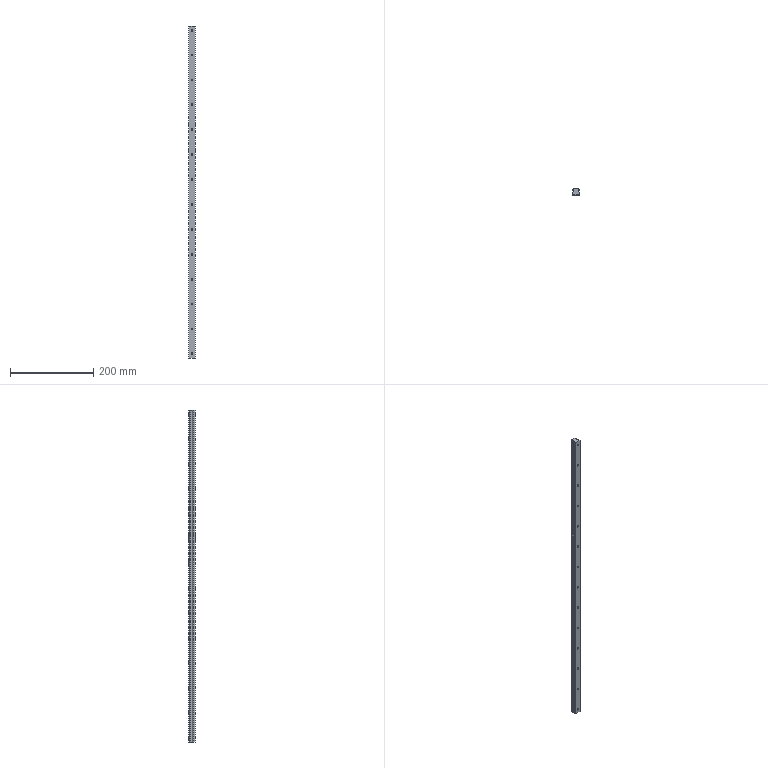Part | SolidWorks | features BaseBody 1 | 1 solid | 96 faces | box 15 x 15 x 800 mm | volume 156317 mm3 | cylinder 62 | plane 34 | commonest cylinder face diameters 4.5 x28 7.5 x28 1.459 x6